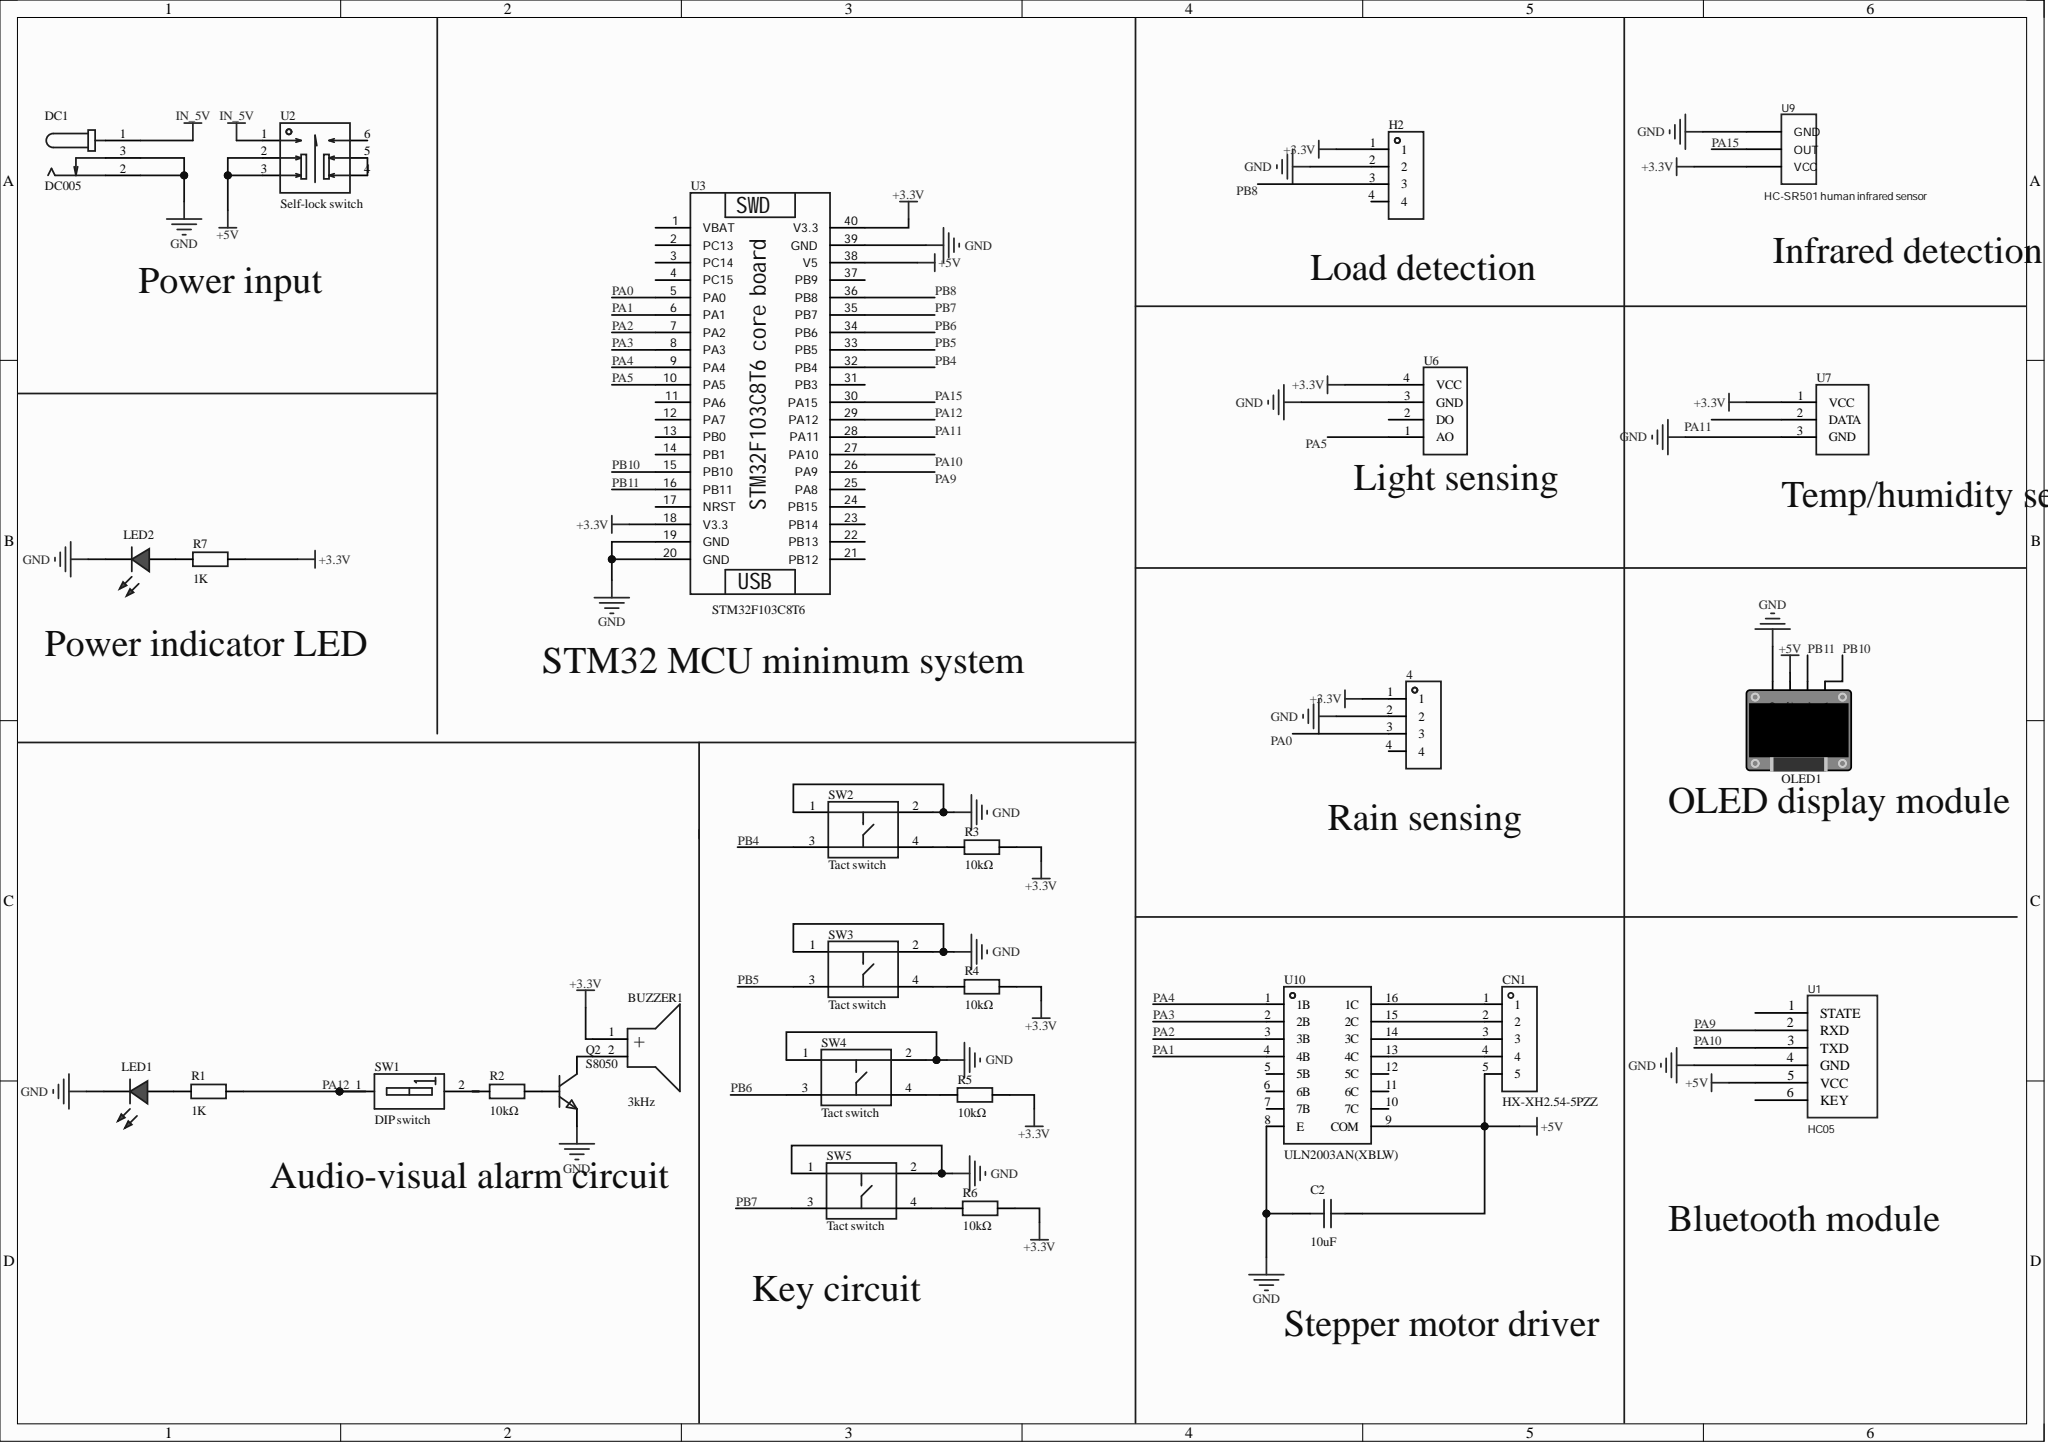Circuit board | Altium Designer | 29 parts | 36 nets
Bill of materials:
Comment,Description,Designator,Footprint,LibRef,Quantity
"","","4, H2","HDR-TH_4P-P2.54-V-F","HDR-F_2.54_1x4P","2"
"3kHz","Drive mode: active (built-in driver circuit); Construction type: electromagnetic; Frequency: 3kHz; Sound pressure (SPL): 85dB;","BUZZER1","BUZZER","HNB09A03","1"
"10uF","","C2","CAP-TH_L10.0-W4.0-P7.50-D0.6-1","ECQU2A224ML","1"
"HX-XH2.54-5PZZ","","CN1","CONN-TH_5P-P2.50_ZX-XH2.54-5PZZ","HX-XH2.54-5PZZ","1"
"DC005","","DC1","DC-IN-TH_DC005","DC005","1"
"","","LED1, LED2","LED-TH_5mm","LED_TH-R_5mm","2"
"","","OLED1","0.96OLED_4P","0.96OLED模块_4P","1"
"S8050","Transistor type: NPN; Collector current (Ic): 500mA; Collector-emitter breakdown voltage (Vceo): 25V; Power dissipation (Pd): 625mW; DC current gain (hFE): 160@50mA,1V;","Q2","TO-92-3_L4.5-W3.5-P1.27-L","S8050_C2931492","1"
"1K","","R1, R7","Res_1/4W","Res_AXIAL-1/4W","2"
"10kΩ","","R2, R3, R4, R5, R6","Res_1/4W","Res_AXIAL-1/4W","5"
"DIP switch","Type: slide, raised; Circuit structure: SPST; Number of positions: 1; Service life: -; Color: red;","SW1","SW-TH_DSWB01LHGET","DSWB01LHGET","1"
"Tact switch","Circuit structure: SPST; Button shape: round button; Actuating force: 2.5N; Mounting: through-hole; Switch length: 6mm; Switch width: 6mm; Switch height: 5mm; Contact current: 50mA; Rated voltage: 12V; With LED: -; Life: 10 ten-thousand cycles;","SW2, SW3, SW4, SW5","KEY-TH_4P-L6.0-W6.0-P4.50-LS6.50","K2-1102DP-C4SW-04","4"
"HC05","","U1","HC05","HC05","1"
"Self-lock switch","Self-lock/no-lock: self-lock;","U2","SW-TH_6P-L5.8-W5.8-P2.00-LS4.5-TR","PB-22E85L","1"
"STM32F103C8T6","","U3","STM32F103C8T6核心板","STM32F103C8T6最小系统板","1"
"","","U6","HDR-TH_4P-P2.54_342-40-104-00-592000","光敏电阻传感器","1"
"","","U7","HDR-TH_3P-P2.54-V-M-B","dth11","1"
"HC-SR501 human infrared sensor","","U9","大闸蟹-HC-SR501人体红外传感器","HC-SR501人体红外传感器","1"
"ULN2003AN(XBLW)","Channels: seven; Collector-emitter breakdown voltage (Vceo): 50V; Collector current (Ic): 500mA;","U10","PDIP-16_L19.3-W6.4-P2.54-LS7.9-BL","ULN2003AN(XBLW)","1"
Netlist (Protel format):
[
4
HDR-TH_4P-P2.54-V-F




]
[
BUZZER1
BUZZER
3kHz



]
[
C2
CAP-TH_L10.0-W4.0-P7.50-D0.6-1
10uF



]
[
CN1
CONN-TH_5P-P2.50_ZX-XH2.54-5PZZ
HX-XH2.54-5PZZ



]
[
DC1
DC-IN-TH_DC005
DC005



]
[
H2
HDR-TH_4P-P2.54-V-F




]
[
LED1
LED-TH_5mm




]
[
LED2
LED-TH_5mm




]
[
OLED1
0.96OLED_4P




]
[
Q2
TO-92-3_L4.5-W3.5-P1.27-L
S8050



]
[
R1
Res_1/4W
1K



]
[
R2
Res_1/4W
10kΩ



]
[
R3
Res_1/4W
10kΩ



]
[
R4
Res_1/4W
10kΩ



]
[
R5
Res_1/4W
10kΩ



]
[
R6
Res_1/4W
10kΩ



]
[
R7
Res_1/4W
1K



]
[
SW1
SW-TH_DSWB01LHGET
DIP switch



]
[
SW2
KEY-TH_4P-L6.0-W6.0-P4.50-LS6.50
Tact switch



]
[
SW3
KEY-TH_4P-L6.0-W6.0-P4.50-LS6.50
Tact switch



]
[
SW4
KEY-TH_4P-L6.0-W6.0-P4.50-LS6.50
Tact switch



]
[
SW5
KEY-TH_4P-L6.0-W6.0-P4.50-LS6.50
Tact switch



]
[
U1
HC05
HC05



]
[
U2
SW-TH_6P-L5.8-W5.8-P2.00-LS4.5-TR
Self-lock switch



]
[
U3
STM32F103C8T6核心板
STM32F103C8T6



]
[
U6
HDR-TH_4P-P2.54_342-40-104-00-592000




]
[
U7
HDR-TH_3P-P2.54-V-M-B




]
[
U9
大闸蟹-HC-SR501人体红外传感器
HC-SR501 human infrared sensor



]
[
U10
PDIP-16_L19.3-W6.4-P2.54-LS7.9-BL
ULN2003AN(XBLW)



]
(
PB11
OLED1-3
U3-16
)
(
PB10
OLED1-4
U3-15
)
(
PB8
H2-3
U3-36
)
(
PB7
SW5-3
U3-35
)
(
PB6
SW4-3
U3-34
)
(
PB5
SW3-3
U3-33
)
(
PB4
SW2-3
U3-32
)
(
PA15
U3-30
U9-2
)
(
PA12
R1-2
SW1-1
U3-29
)
(
PA11
U3-28
U7-2
)
(
PA10
U1-3
U3-27
)
(
PA9
U1-2
U3-26
)
(
PA5
U3-10
U6-1
)
(
PA4
U3-9
U10-1
)
(
PA3
U3-8
U10-2
)
(
PA2
U3-7
U10-3
)
(
PA1
U3-6
U10-4
)
(
PA0
4-3
U3-5
)
(
NetU2_4
U2-4
U2-5
)
(
NetR6_1
R6-1
SW5-4
)
(
NetR5_1
R5-1
SW4-4
)
(
NetR4_1
R4-1
SW3-4
)
(
NetR3_1
R3-1
SW2-4
)
(
NetR2_1
R2-1
SW1-2
)
(
NetQ2_2
Q2-2
R2-2
)
(
NetLED2_1
LED2-1
R7-1
)
(
NetLED1_1
LED1-1
R1-1
)
(
NetCN1_4
CN1-4
U10-13
)
(
NetCN1_3
CN1-3
U10-14
)
(
NetCN1_2
CN1-2
U10-15
)
(
NetCN1_1
CN1-1
U10-16
)
(
NetBUZZER1_2
BUZZER1-2
Q2-3
)
(
IN_5V
DC1-1
U2-1
)
(
GND
4-2
C2-1
DC1-2
DC1-3
H2-2
LED1-2
LED2-2
OLED1-1
Q2-1
SW2-1
SW2-2
SW3-1
SW3-2
SW4-1
SW4-2
SW5-1
SW5-2
U1-4
U3-19
U3-20
U3-39
U6-3
U7-3
U9-1
U10-8
)
(
+5V
C2-2
CN1-5
OLED1-2
U1-5
U2-2
U2-3
U3-38
U10-9
)
(
+3.3V
4-1
BUZZER1-1
H2-1
R3-2
R4-2
R5-2
R6-2
R7-2
U3-18
U3-40
U6-4
U7-1
U9-3
)